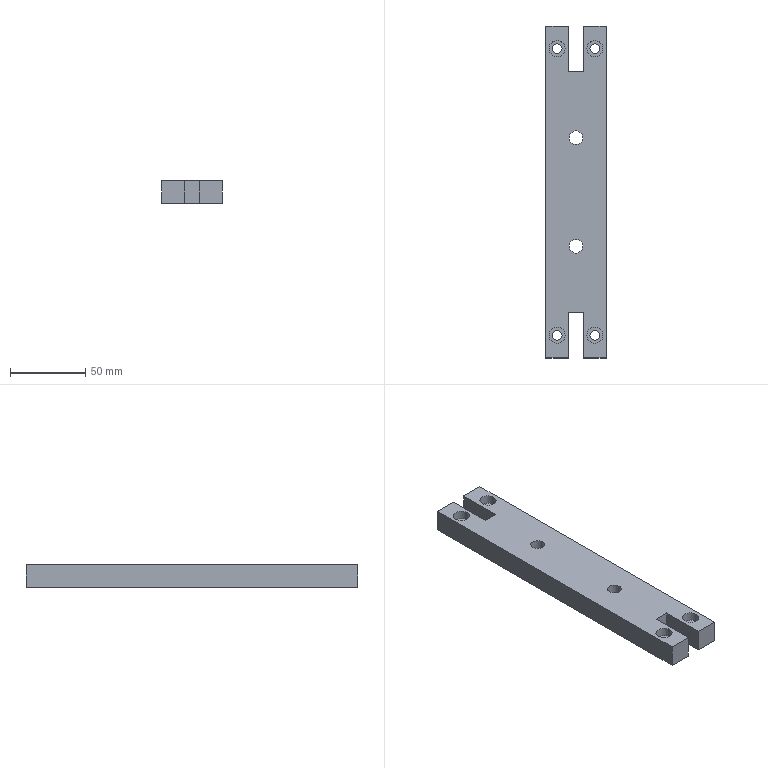Part | STEP file | YBQDJ-PD-18 | 1 solid | 28 faces | box 40 x 220 x 15 mm | volume 117739 mm3 | plane 18 | cylinder 10 | commonest cylinder face diameters 6.5 x4 10.7 x4 9 x2